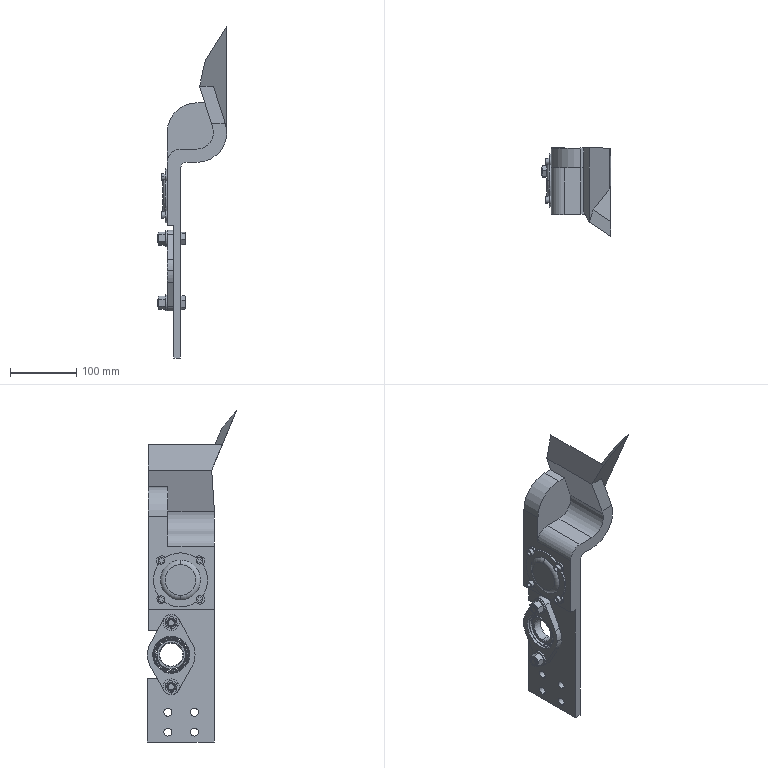Part | SolidWorks | 15 solids | 1100 faces | box 105 x 134.847 x 502.101 mm | volume 897409 mm3 | cone 378 | cylinder 245 | plane 189 | sphere 176 | torus 112 | commonest cylinder face diameters 6 x128 12 x24 62 x10 5 x8 10 x8 43.3 x8